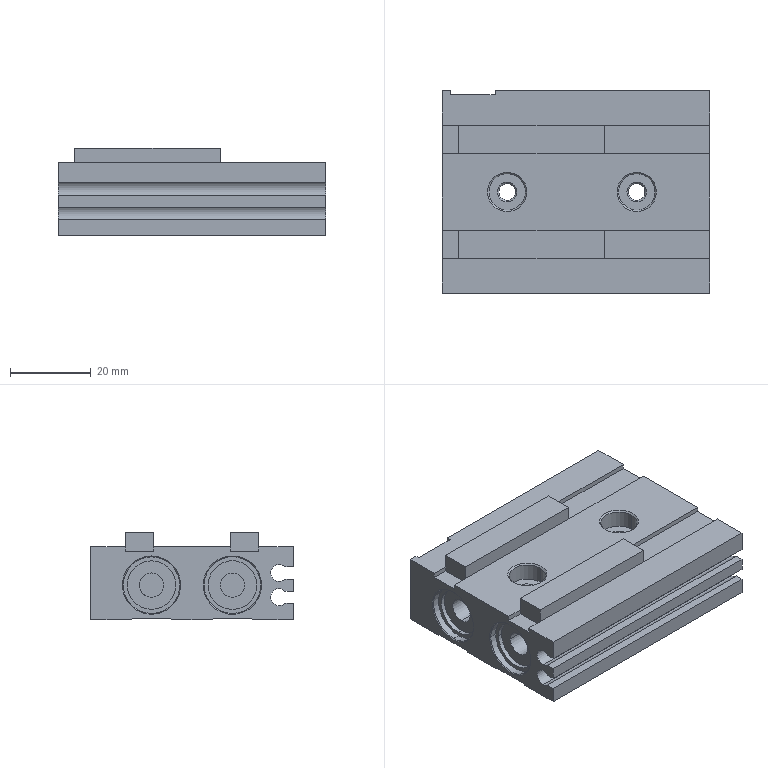Part | SolidWorks | features BaseBody 1 | 1 solid | 177 faces | box 66 x 50 x 21.5 mm | volume 44662 mm3 | plane 70 | cylinder 63 | cone 44 | commonest cylinder face diameters 3.242 x12 12 x12 4.134 x8 14 x8 4.2 x6 4 x5